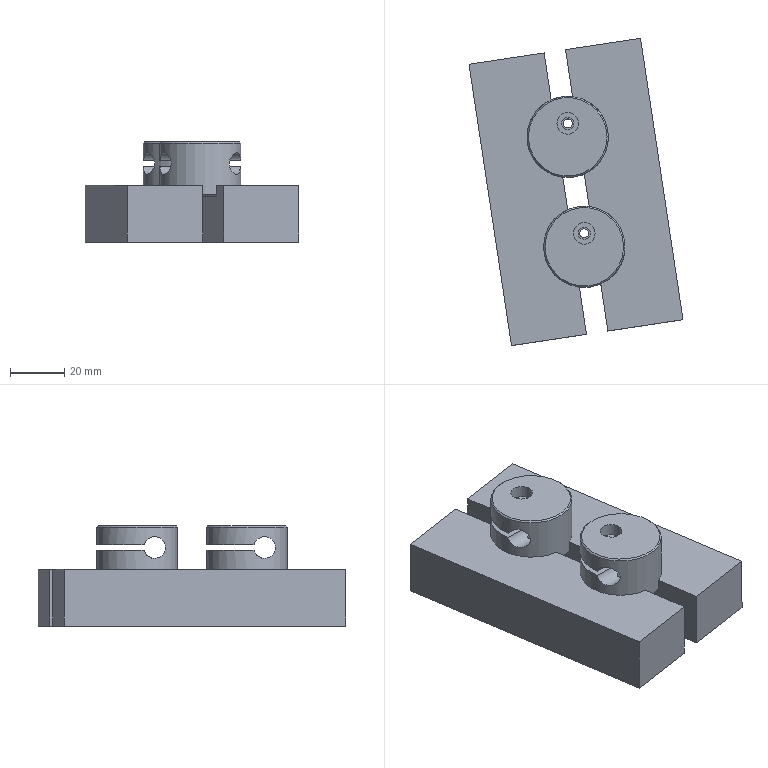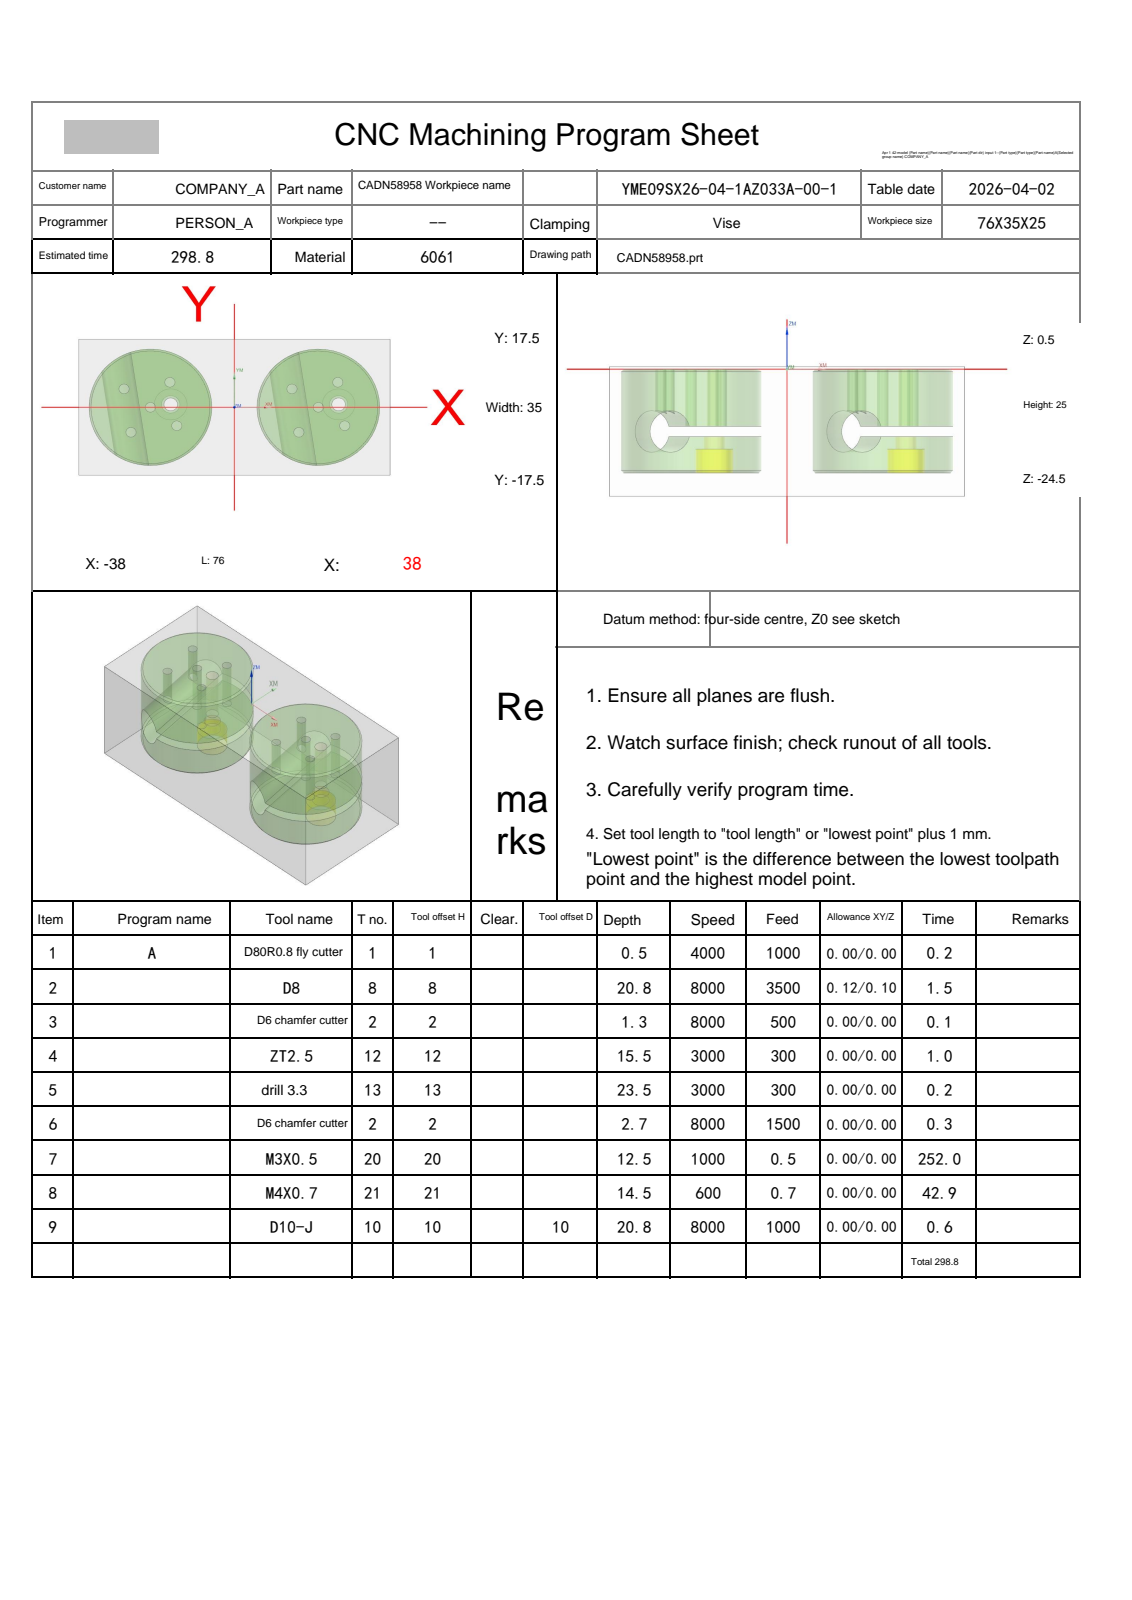NC program | NX | posted by the shop | part box 78.946 x 113.372 x 37 mm
Lines 2155 to 2409 of 2409:
N3 T02 M06
(D6 chamfer cutter  D=6. R=0. H=02 ce=0.00 di=0.10)
G00 G90 G54 X-25.25 Y-6.437 M03 S8000
G43 H02 Z20.
M08
G98 G81 X-25.25 Y-6.437 Z-.8 R1. F500.
X-26.937 Y4.75
X-20.5 Y0.0
X-15.75 Y6.437
X-15.556 Y.746
X-14.063 Y-4.75
X14.063 Y4.75
X25.25 Y6.437
X25.444 Y.746
X26.937 Y-4.75
X20.5 Y0.0
X15.75 Y-6.437
G80
G00 Z20.
G91 G28 Z0.0
M05
M09
G91 G28 Z0.0
M01
N4 T12 M06
(ZT2.5 D=2.5 DR_a=118 H=12)
G00 G90 G54 X-15.75 Y6.437 M03 S3000
G43 H12 Z20.
M08
G98 G83 X-15.75 Y6.437 Z-14.5 R1. F300. Q2.
X-20.5 Y0.0
X-14.063 Y-4.75
X20.5 Y0.0
X26.937 Y-4.75
X25.25 Y6.437
G80
G00 Z20.
G00 G90 X-26.937 Y4.75 M03 S3000
Z20.
G98 G83 X-26.937 Y4.75 Z-15. R1. F100. Q2.
X-25.25 Y-6.437
X14.063 Y4.75
X15.75 Y-6.437
G80
G00 Z20.
G91 G28 Z0.0
M05
M09
G91 G28 Z0.0
M01
N5 T13 M06
(drill 3.3 D=3.3 DR_a=118 H=13)
G00 G90 G54 X-15.556 Y.746 M03 S3000
G43 H13 Z20.
M08
G98 G83 X-15.556 Y.746 Z-23. R1. F300. Q2.
X25.444
G80
G00 Z20.
G91 G28 Z0.0
M05
M09
G91 G28 Z0.0
M01
N6 T02 M06
(D6 chamfer cutter  D=6. R=0. H=02 ce=0.00 di=0.10)
G00 G90 G54 X-25.25 Y-6.437 M03 S8000
G43 H02 Z20.
M08
G98 G81 X-25.25 Y-6.437 Z-1.75 R3. F500.
X-26.937 Y4.75
X-20.5 Y0.0
X-15.75 Y6.437
X-14.063 Y-4.75
X14.063 Y4.75
X20.5 Y0.0
X25.25 Y6.437
X26.937 Y-4.75
X15.75 Y-6.437
G80
G00 Z20.
G00 G90 X-15.556 Y.746 M03 S8000
Z20.
G98 G81 X-15.556 Y.746 Z-2.2 R3. F500.
X25.444
G80
G00 Z20.
G00 G90 X-24.2 Y16.49 M03 S6500
Z20.
Z.3
G01 Z-1.2 F1500.
G03 X-23.021 Y15.511 I1.179 J.221
G01 X-22.842 Y15.524
G02 X-20.5 Y15.7 I2.342 J-15.524
X-4.8 Y0.0 I0.0 J-15.7
X-20.5 Y-15.7 I-15.7 J0.0
X-36.2 Y0.0 I0.0 J15.7
X-22.842 Y15.524 I15.7 J0.0
X-22.446 Y15.579 I2.342 J-15.524
G03 X-21.394 Y16.77 I-.149 J1.191
G01 X-21.399 Y16.876
Z.3
G00 Z20.
X24.2 Y-16.49
Z.3
G01 Z-1.2
G03 X23.021 Y-15.511 I-1.179 J-.221
G01 X22.842 Y-15.524
G02 X20.5 Y-15.7 I-2.342 J15.524
X4.8 Y0.0 I0.0 J15.7
X13.787 Y14.192 I15.7 J0.0
X14.007 Y14.294 I6.713 J-14.192
X18.076 Y15.512 I6.493 J-14.294
G01 X18.158 Y15.524
G02 X20.5 Y15.7 I2.342 J-15.524
X36.2 Y0.0 I0.0 J-15.7
X22.842 Y-15.524 I-15.7 J0.0
X22.446 Y-15.579 I-2.342 J15.524
G03 X21.394 Y-16.77 I.149 J-1.191
G01 X21.399 Y-16.876
Z.3
G00 Z20.
G91 G28 Z0.0
M05
M09
G91 G28 Z0.0
M01
N7 T20 M06
(M3X0.5 D=2.5 DR_a=180 H=20)
G00 G90 G54 X-26.937 Y4.75 M03 S1000
G43 H20 Z20.
M08
G95
G98 G84 X-26.937 Y4.75 Z-11. R1. F.5 Q2.
X-25.25 Y-6.437
X14.063 Y4.75
X15.75 Y-6.437
G80
G94
G00 Z20.
G00 G90 X-15.75 Y6.437 M03 S800
Z20.
G95
G98 G84 X-15.75 Y6.437 Z-12. R1. F.5 Q5.
X-20.5 Y0.0
X-14.063 Y-4.75
X20.5 Y0.0
X26.937 Y-4.75
X25.25 Y6.437
G80
G94
G00 Z20.
G91 G28 Z0.0
M05
M09
G91 G28 Z0.0
M01
N8 T21 M06
(M4X0.7 D=3.3 DR_a=180 H=21)
G00 G90 G54 X-15.556 Y.746 M03 S600
G43 H21 Z20.
M08
G95
G98 G84 X-15.556 Y.746 Z-14. R1. F.7 Q4.
X25.444
G80
G94
G00 Z20.
G91 G28 Z0.0
M05
M09
G91 G28 Z0.0
M01
N9 T10 M06
(D10-J  D=10. R=0. H=10 ce=0.00 di=0.00)
G00 G90 G54 X24.652 Y-20.789 M03 S8000
G43 H10 Z20.
M08
Z-9.65
G01 Z-10.15 F1000.
G41 D10
X24.617 Y-20.592
G03 X23.632 Y-19.765 I-.985 J-.173
G01 X23.483 Y-19.776
G02 X20.5 Y-20. I-2.983 J19.776
X.5 Y0.0 I0.0 J20.
X20.5 Y20. I20. J0.0
X40.5 Y0.0 I0.0 J-20.
X23.483 Y-19.776 I-20. J0.0
X22.988 Y-19.845 I-2.983 J19.776
G03 X22.112 Y-20.837 I.124 J-.992
G01 X22.117 Y-20.938
G40 X22.138 Y-21.137
Z-9.65
G00 Z20.
X-16.348 Y-20.789
Z-9.65
G01 Z-10.15
G41 D10
X-16.383 Y-20.592
G03 X-17.368 Y-19.765 I-.985 J-.173
G01 X-17.517 Y-19.776
G02 X-20.5 Y-20. I-2.983 J19.776
X-40.5 Y0.0 I0.0 J20.
X-20.5 Y20. I20. J0.0
X-.5 Y0.0 I0.0 J-20.
X-17.517 Y-19.776 I-20. J0.0
X-18.012 Y-19.845 I-2.983 J19.776
G03 X-18.888 Y-20.837 I.124 J-.992
G01 X-18.883 Y-20.938
G40 X-18.862 Y-21.137
Z-9.65
G00 Z20.
X-16.348 Y-20.789
Z-19.8
G01 Z-20.3
G41 D10
X-16.383 Y-20.592
G03 X-17.368 Y-19.765 I-.985 J-.173
G01 X-17.517 Y-19.776
G02 X-20.5 Y-20. I-2.983 J19.776
X-40.5 Y0.0 I0.0 J20.
X-20.5 Y20. I20. J0.0
X-.5 Y0.0 I0.0 J-20.
X-17.517 Y-19.776 I-20. J0.0
X-18.012 Y-19.845 I-2.983 J19.776
G03 X-18.888 Y-20.837 I.124 J-.992
G01 X-18.883 Y-20.938
G40 X-18.862 Y-21.137
Z-19.8
G00 Z20.
X24.652 Y-20.789
Z-19.8
G01 Z-20.3
G41 D10
X24.617 Y-20.592
G03 X23.632 Y-19.765 I-.985 J-.173
G01 X23.483 Y-19.776
G02 X20.5 Y-20. I-2.983 J19.776
X.5 Y0.0 I0.0 J20.
X20.5 Y20. I20. J0.0
X40.5 Y0.0 I0.0 J-20.
X23.483 Y-19.776 I-20. J0.0
X22.988 Y-19.845 I-2.983 J19.776
G03 X22.112 Y-20.837 I.124 J-.992
G01 X22.117 Y-20.938
G40 X22.138 Y-21.137
Z-19.8
G00 Z20.
M05
M09
G91 G28 Z0.0
G91 G28 Y0.0
M30
%